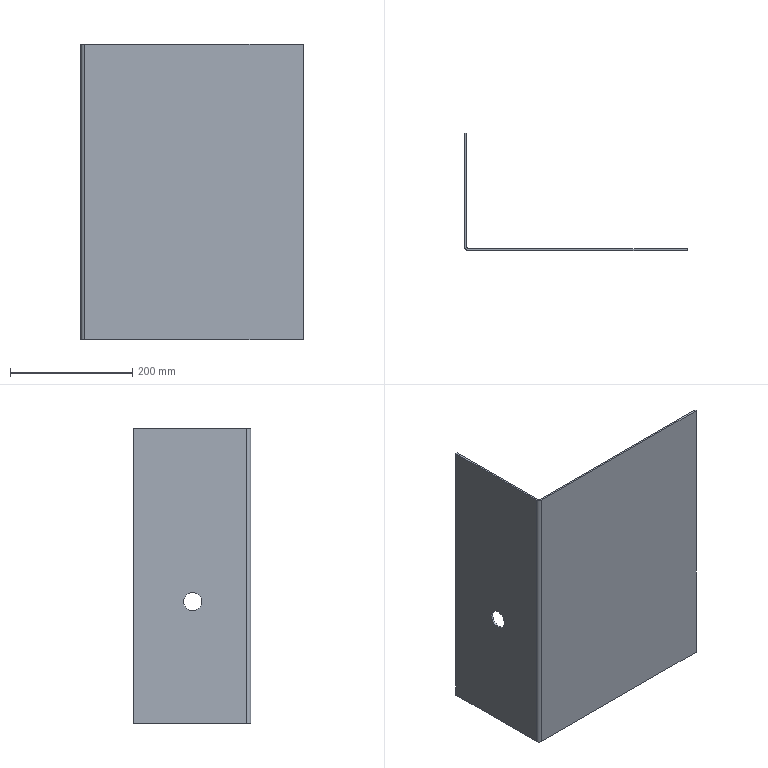Part | SolidWorks | features Cut 1, FlatPattern 1, SMBaseFlange 1, SheetMetal 1 | 1 solid | 16 faces | box 364 x 192 x 484 mm | volume 798031 mm3 | plane 12 | cylinder 4 | commonest cylinder face diameters 30 x2 6 x1 12 x1
STEP:
#1=CARTESIAN_POINT('',(3.,95.,215.));
#2=VERTEX_POINT('',#1);
#3=CARTESIAN_POINT('',(3.,95.,185.));
#4=VERTEX_POINT('',#3);
#5=CARTESIAN_POINT('',(3.,95.,200.));
#6=DIRECTION('',(1.,0.,0.));
#7=DIRECTION('',(0.,0.,-1.));
#8=AXIS2_PLACEMENT_3D('',#5,#6,#7);
#9=CIRCLE('',#8,15.);
#10=EDGE_CURVE('',#2,#4,#9,.T.);
#11=ORIENTED_EDGE('',*,*,#10,.T.);
#12=CARTESIAN_POINT('',(0.,95.,185.));
#13=VERTEX_POINT('',#12);
#14=CARTESIAN_POINT('',(10.,95.,185.));
#15=DIRECTION('',(-1.,0.,0.));
#16=VECTOR('',#15,1000.);
#17=LINE('',#14,#16);
#18=EDGE_CURVE('',#4,#13,#17,.T.);
#19=ORIENTED_EDGE('',*,*,#18,.T.);
#20=CARTESIAN_POINT('',(0.,95.,215.));
#21=VERTEX_POINT('',#20);
#22=CARTESIAN_POINT('',(0.,95.,200.));
#23=DIRECTION('',(-1.,0.,0.));
#24=DIRECTION('',(0.,0.,1.));
#25=AXIS2_PLACEMENT_3D('',#22,#23,#24);
#26=CIRCLE('',#25,15.);
#27=EDGE_CURVE('',#13,#21,#26,.T.);
#28=ORIENTED_EDGE('',*,*,#27,.T.);
#29=CARTESIAN_POINT('',(10.,95.,215.));
#30=DIRECTION('',(-1.,0.,0.));
#31=VECTOR('',#30,1000.);
#32=LINE('',#29,#31);
#33=EDGE_CURVE('',#2,#21,#32,.T.);
#34=ORIENTED_EDGE('',*,*,#33,.F.);
#35=EDGE_LOOP('',(#11,#19,#28,#34));
#36=FACE_OUTER_BOUND('',#35,.T.);
#37=CARTESIAN_POINT('',(10.,95.,200.));
#38=DIRECTION('',(-1.,0.,0.));
#39=DIRECTION('',(0.,0.,1.));
#40=AXIS2_PLACEMENT_3D('',#37,#38,#39);
#41=CYLINDRICAL_SURFACE('',#40,15.);
#42=ADVANCED_FACE('',(#36),#41,.F.);
#43=CARTESIAN_POINT('',(0.,6.,484.));
#44=VERTEX_POINT('',#43);
#45=CARTESIAN_POINT('',(3.,6.,484.));
#46=VERTEX_POINT('',#45);
#47=CARTESIAN_POINT('',(0.,6.,484.));
#48=DIRECTION('',(1.,0.,0.));
#49=VECTOR('',#48,1000.);
#50=LINE('',#47,#49);
#51=EDGE_CURVE('',#44,#46,#50,.T.);
#52=ORIENTED_EDGE('',*,*,#51,.F.);
#53=CARTESIAN_POINT('',(6.,0.,484.));
#54=VERTEX_POINT('',#53);
#55=CARTESIAN_POINT('',(6.,6.,484.));
#56=DIRECTION('',(0.,0.,1.));
#57=DIRECTION('',(-1.,0.,0.));
#58=AXIS2_PLACEMENT_3D('',#55,#56,#57);
#59=CIRCLE('',#58,6.);
#60=EDGE_CURVE('',#44,#54,#59,.T.);
#61=ORIENTED_EDGE('',*,*,#60,.T.);
#62=CARTESIAN_POINT('',(6.,3.,484.));
#63=VERTEX_POINT('',#62);
#64=CARTESIAN_POINT('',(6.,3.,484.));
#65=DIRECTION('',(0.,-1.,0.));
#66=VECTOR('',#65,1000.);
#67=LINE('',#64,#66);
#68=EDGE_CURVE('',#63,#54,#67,.T.);
#69=ORIENTED_EDGE('',*,*,#68,.F.);
#70=CARTESIAN_POINT('',(6.,6.,484.));
#71=DIRECTION('',(0.,0.,1.));
#72=DIRECTION('',(1.,0.,0.));
#73=AXIS2_PLACEMENT_3D('',#70,#71,#72);
#74=CIRCLE('',#73,3.);
#75=EDGE_CURVE('',#46,#63,#74,.T.);
#76=ORIENTED_EDGE('',*,*,#75,.F.);
#77=EDGE_LOOP('',(#52,#61,#69,#76));
#78=FACE_OUTER_BOUND('',#77,.T.);
#79=CARTESIAN_POINT('',(0.,6.,484.));
#80=DIRECTION('',(0.,0.,1.));
#81=DIRECTION('',(1.,0.,0.));
#82=AXIS2_PLACEMENT_3D('',#79,#80,#81);
#83=PLANE('',#82);
#84=ADVANCED_FACE('',(#78),#83,.T.);
#85=CARTESIAN_POINT('',(0.,192.,484.));
#86=VERTEX_POINT('',#85);
#87=CARTESIAN_POINT('',(0.,0.,484.));
#88=DIRECTION('',(0.,-1.,0.));
#89=VECTOR('',#88,1000.);
#90=LINE('',#87,#89);
#91=EDGE_CURVE('',#86,#44,#90,.T.);
#92=ORIENTED_EDGE('',*,*,#91,.T.);
#93=ORIENTED_EDGE('',*,*,#51,.T.);
#94=CARTESIAN_POINT('',(3.,192.,484.));
#95=VERTEX_POINT('',#94);
#96=CARTESIAN_POINT('',(3.,0.,484.));
#97=DIRECTION('',(0.,-1.,0.));
#98=VECTOR('',#97,1000.);
#99=LINE('',#96,#98);
#100=EDGE_CURVE('',#95,#46,#99,.T.);
#101=ORIENTED_EDGE('',*,*,#100,.F.);
#102=CARTESIAN_POINT('',(0.,192.,484.));
#103=DIRECTION('',(1.,0.,0.));
#104=VECTOR('',#103,1000.);
#105=LINE('',#102,#104);
#106=EDGE_CURVE('',#86,#95,#105,.T.);
#107=ORIENTED_EDGE('',*,*,#106,.F.);
#108=EDGE_LOOP('',(#92,#93,#101,#107));
#109=FACE_OUTER_BOUND('',#108,.T.);
#110=CARTESIAN_POINT('',(6.,3.,484.));
#111=DIRECTION('',(0.,0.,1.));
#112=DIRECTION('',(1.,0.,0.));
#113=AXIS2_PLACEMENT_3D('',#110,#111,#112);
#114=PLANE('',#113);
#115=ADVANCED_FACE('',(#109),#114,.T.);
#116=CARTESIAN_POINT('',(6.,0.,0.));
#117=VERTEX_POINT('',#116);
#118=CARTESIAN_POINT('',(6.,3.,0.));
#119=VERTEX_POINT('',#118);
#120=CARTESIAN_POINT('',(6.,0.,0.));
#121=DIRECTION('',(0.,1.,0.));
#122=VECTOR('',#121,1000.);
#123=LINE('',#120,#122);
#124=EDGE_CURVE('',#117,#119,#123,.T.);
#125=ORIENTED_EDGE('',*,*,#124,.F.);
#126=CARTESIAN_POINT('',(0.,6.,0.));
#127=VERTEX_POINT('',#126);
#128=CARTESIAN_POINT('',(6.,6.,0.));
#129=DIRECTION('',(0.,0.,1.));
#130=DIRECTION('',(-1.,0.,0.));
#131=AXIS2_PLACEMENT_3D('',#128,#129,#130);
#132=CIRCLE('',#131,6.);
#133=EDGE_CURVE('',#127,#117,#132,.T.);
#134=ORIENTED_EDGE('',*,*,#133,.F.);
#135=CARTESIAN_POINT('',(3.,6.,0.));
#136=VERTEX_POINT('',#135);
#137=CARTESIAN_POINT('',(3.,6.,0.));
#138=DIRECTION('',(-1.,0.,0.));
#139=VECTOR('',#138,1000.);
#140=LINE('',#137,#139);
#141=EDGE_CURVE('',#136,#127,#140,.T.);
#142=ORIENTED_EDGE('',*,*,#141,.F.);
#143=CARTESIAN_POINT('',(6.,6.,0.));
#144=DIRECTION('',(0.,0.,1.));
#145=DIRECTION('',(1.,0.,0.));
#146=AXIS2_PLACEMENT_3D('',#143,#144,#145);
#147=CIRCLE('',#146,3.);
#148=EDGE_CURVE('',#136,#119,#147,.T.);
#149=ORIENTED_EDGE('',*,*,#148,.T.);
#150=EDGE_LOOP('',(#125,#134,#142,#149));
#151=FACE_OUTER_BOUND('',#150,.T.);
#152=CARTESIAN_POINT('',(6.,0.,0.));
#153=DIRECTION('',(0.,0.,-1.));
#154=DIRECTION('',(-1.,0.,0.));
#155=AXIS2_PLACEMENT_3D('',#152,#153,#154);
#156=PLANE('',#155);
#157=ADVANCED_FACE('',(#151),#156,.T.);
#158=CARTESIAN_POINT('',(364.,0.,0.));
#159=VERTEX_POINT('',#158);
#160=CARTESIAN_POINT('',(0.,0.,0.));
#161=DIRECTION('',(1.,0.,0.));
#162=VECTOR('',#161,1000.);
#163=LINE('',#160,#162);
#164=EDGE_CURVE('',#117,#159,#163,.T.);
#165=ORIENTED_EDGE('',*,*,#164,.F.);
#166=ORIENTED_EDGE('',*,*,#124,.T.);
#167=CARTESIAN_POINT('',(364.,3.,0.));
#168=VERTEX_POINT('',#167);
#169=CARTESIAN_POINT('',(0.,3.,0.));
#170=DIRECTION('',(1.,0.,0.));
#171=VECTOR('',#170,1000.);
#172=LINE('',#169,#171);
#173=EDGE_CURVE('',#119,#168,#172,.T.);
#174=ORIENTED_EDGE('',*,*,#173,.T.);
#175=CARTESIAN_POINT('',(364.,3.,0.));
#176=DIRECTION('',(0.,-1.,0.));
#177=VECTOR('',#176,1000.);
#178=LINE('',#175,#177);
#179=EDGE_CURVE('',#168,#159,#178,.T.);
#180=ORIENTED_EDGE('',*,*,#179,.T.);
#181=EDGE_LOOP('',(#165,#166,#174,#180));
#182=FACE_OUTER_BOUND('',#181,.T.);
#183=CARTESIAN_POINT('',(3.,6.,0.));
#184=DIRECTION('',(0.,0.,-1.));
#185=DIRECTION('',(-1.,0.,0.));
#186=AXIS2_PLACEMENT_3D('',#183,#184,#185);
#187=PLANE('',#186);
#188=ADVANCED_FACE('',(#182),#187,.T.);
#189=ORIENTED_EDGE('',*,*,#164,.T.);
#190=CARTESIAN_POINT('',(364.,0.,484.));
#191=VERTEX_POINT('',#190);
#192=CARTESIAN_POINT('',(364.,0.,484.));
#193=DIRECTION('',(0.,0.,-1.));
#194=VECTOR('',#193,1000.);
#195=LINE('',#192,#194);
#196=EDGE_CURVE('',#191,#159,#195,.T.);
#197=ORIENTED_EDGE('',*,*,#196,.F.);
#198=CARTESIAN_POINT('',(0.,0.,484.));
#199=DIRECTION('',(1.,0.,0.));
#200=VECTOR('',#199,1000.);
#201=LINE('',#198,#200);
#202=EDGE_CURVE('',#54,#191,#201,.T.);
#203=ORIENTED_EDGE('',*,*,#202,.F.);
#204=CARTESIAN_POINT('',(6.,0.,484.));
#205=DIRECTION('',(0.,0.,-1.));
#206=VECTOR('',#205,1000.);
#207=LINE('',#204,#206);
#208=EDGE_CURVE('',#54,#117,#207,.T.);
#209=ORIENTED_EDGE('',*,*,#208,.T.);
#210=EDGE_LOOP('',(#189,#197,#203,#209));
#211=FACE_OUTER_BOUND('',#210,.T.);
#212=CARTESIAN_POINT('',(0.,0.,484.));
#213=DIRECTION('',(0.,1.,0.));
#214=DIRECTION('',(0.,0.,1.));
#215=AXIS2_PLACEMENT_3D('',#212,#213,#214);
#216=PLANE('',#215);
#217=ADVANCED_FACE('',(#211),#216,.F.);
#218=ORIENTED_EDGE('',*,*,#179,.F.);
#219=CARTESIAN_POINT('',(364.,3.,484.));
#220=VERTEX_POINT('',#219);
#221=CARTESIAN_POINT('',(364.,3.,484.));
#222=DIRECTION('',(0.,0.,-1.));
#223=VECTOR('',#222,1000.);
#224=LINE('',#221,#223);
#225=EDGE_CURVE('',#220,#168,#224,.T.);
#226=ORIENTED_EDGE('',*,*,#225,.F.);
#227=CARTESIAN_POINT('',(364.,3.,484.));
#228=DIRECTION('',(0.,-1.,0.));
#229=VECTOR('',#228,1000.);
#230=LINE('',#227,#229);
#231=EDGE_CURVE('',#220,#191,#230,.T.);
#232=ORIENTED_EDGE('',*,*,#231,.T.);
#233=ORIENTED_EDGE('',*,*,#196,.T.);
#234=EDGE_LOOP('',(#218,#226,#232,#233));
#235=FACE_OUTER_BOUND('',#234,.T.);
#236=CARTESIAN_POINT('',(364.,3.,484.));
#237=DIRECTION('',(1.,0.,0.));
#238=DIRECTION('',(0.,0.,-1.));
#239=AXIS2_PLACEMENT_3D('',#236,#237,#238);
#240=PLANE('',#239);
#241=ADVANCED_FACE('',(#235),#240,.T.);
#242=ORIENTED_EDGE('',*,*,#173,.F.);
#243=CARTESIAN_POINT('',(6.,3.,484.));
#244=DIRECTION('',(0.,0.,-1.));
#245=VECTOR('',#244,1000.);
#246=LINE('',#243,#245);
#247=EDGE_CURVE('',#63,#119,#246,.T.);
#248=ORIENTED_EDGE('',*,*,#247,.F.);
#249=CARTESIAN_POINT('',(0.,3.,484.));
#250=DIRECTION('',(1.,0.,0.));
#251=VECTOR('',#250,1000.);
#252=LINE('',#249,#251);
#253=EDGE_CURVE('',#63,#220,#252,.T.);
#254=ORIENTED_EDGE('',*,*,#253,.T.);
#255=ORIENTED_EDGE('',*,*,#225,.T.);
#256=EDGE_LOOP('',(#242,#248,#254,#255));
#257=FACE_OUTER_BOUND('',#256,.T.);
#258=CARTESIAN_POINT('',(0.,3.,484.));
#259=DIRECTION('',(0.,1.,0.));
#260=DIRECTION('',(0.,0.,1.));
#261=AXIS2_PLACEMENT_3D('',#258,#259,#260);
#262=PLANE('',#261);
#263=ADVANCED_FACE('',(#257),#262,.T.);
#264=ORIENTED_EDGE('',*,*,#148,.F.);
#265=CARTESIAN_POINT('',(3.,6.,484.));
#266=DIRECTION('',(0.,0.,-1.));
#267=VECTOR('',#266,1000.);
#268=LINE('',#265,#267);
#269=EDGE_CURVE('',#46,#136,#268,.T.);
#270=ORIENTED_EDGE('',*,*,#269,.F.);
#271=ORIENTED_EDGE('',*,*,#75,.T.);
#272=ORIENTED_EDGE('',*,*,#247,.T.);
#273=EDGE_LOOP('',(#264,#270,#271,#272));
#274=FACE_OUTER_BOUND('',#273,.T.);
#275=CARTESIAN_POINT('',(6.,6.,484.));
#276=DIRECTION('',(0.,0.,-1.));
#277=DIRECTION('',(-1.,0.,0.));
#278=AXIS2_PLACEMENT_3D('',#275,#276,#277);
#279=CYLINDRICAL_SURFACE('',#278,3.);
#280=ADVANCED_FACE('',(#274),#279,.F.);
#281=ORIENTED_EDGE('',*,*,#10,.F.);
#282=CARTESIAN_POINT('',(3.,95.,200.));
#283=DIRECTION('',(1.,0.,0.));
#284=DIRECTION('',(0.,0.,-1.));
#285=AXIS2_PLACEMENT_3D('',#282,#283,#284);
#286=CIRCLE('',#285,15.);
#287=EDGE_CURVE('',#4,#2,#286,.T.);
#288=ORIENTED_EDGE('',*,*,#287,.F.);
#289=EDGE_LOOP('',(#281,#288));
#290=FACE_BOUND('',#289,.T.);
#291=CARTESIAN_POINT('',(3.,192.,0.));
#292=VERTEX_POINT('',#291);
#293=CARTESIAN_POINT('',(3.,0.,0.));
#294=DIRECTION('',(0.,-1.,0.));
#295=VECTOR('',#294,1000.);
#296=LINE('',#293,#295);
#297=EDGE_CURVE('',#292,#136,#296,.T.);
#298=ORIENTED_EDGE('',*,*,#297,.F.);
#299=CARTESIAN_POINT('',(3.,192.,484.));
#300=DIRECTION('',(0.,0.,-1.));
#301=VECTOR('',#300,1000.);
#302=LINE('',#299,#301);
#303=EDGE_CURVE('',#95,#292,#302,.T.);
#304=ORIENTED_EDGE('',*,*,#303,.F.);
#305=ORIENTED_EDGE('',*,*,#100,.T.);
#306=ORIENTED_EDGE('',*,*,#269,.T.);
#307=EDGE_LOOP('',(#298,#304,#305,#306));
#308=FACE_OUTER_BOUND('',#307,.T.);
#309=CARTESIAN_POINT('',(3.,0.,484.));
#310=DIRECTION('',(1.,0.,0.));
#311=DIRECTION('',(0.,0.,-1.));
#312=AXIS2_PLACEMENT_3D('',#309,#310,#311);
#313=PLANE('',#312);
#314=ADVANCED_FACE('',(#290,#308),#313,.T.);
#315=CARTESIAN_POINT('',(0.,192.,0.));
#316=VERTEX_POINT('',#315);
#317=CARTESIAN_POINT('',(0.,192.,0.));
#318=DIRECTION('',(1.,0.,0.));
#319=VECTOR('',#318,1000.);
#320=LINE('',#317,#319);
#321=EDGE_CURVE('',#316,#292,#320,.T.);
#322=ORIENTED_EDGE('',*,*,#321,.F.);
#323=CARTESIAN_POINT('',(0.,192.,484.));
#324=DIRECTION('',(0.,0.,-1.));
#325=VECTOR('',#324,1000.);
#326=LINE('',#323,#325);
#327=EDGE_CURVE('',#86,#316,#326,.T.);
#328=ORIENTED_EDGE('',*,*,#327,.F.);
#329=ORIENTED_EDGE('',*,*,#106,.T.);
#330=ORIENTED_EDGE('',*,*,#303,.T.);
#331=EDGE_LOOP('',(#322,#328,#329,#330));
#332=FACE_OUTER_BOUND('',#331,.T.);
#333=CARTESIAN_POINT('',(0.,192.,484.));
#334=DIRECTION('',(0.,1.,0.));
#335=DIRECTION('',(0.,0.,1.));
#336=AXIS2_PLACEMENT_3D('',#333,#334,#335);
#337=PLANE('',#336);
#338=ADVANCED_FACE('',(#332),#337,.T.);
#339=CARTESIAN_POINT('',(0.,95.,200.));
#340=DIRECTION('',(-1.,0.,0.));
#341=DIRECTION('',(0.,0.,1.));
#342=AXIS2_PLACEMENT_3D('',#339,#340,#341);
#343=CIRCLE('',#342,15.);
#344=EDGE_CURVE('',#21,#13,#343,.T.);
#345=ORIENTED_EDGE('',*,*,#344,.F.);
#346=ORIENTED_EDGE('',*,*,#27,.F.);
#347=EDGE_LOOP('',(#345,#346));
#348=FACE_BOUND('',#347,.T.);
#349=CARTESIAN_POINT('',(0.,0.,0.));
#350=DIRECTION('',(0.,-1.,0.));
#351=VECTOR('',#350,1000.);
#352=LINE('',#349,#351);
#353=EDGE_CURVE('',#316,#127,#352,.T.);
#354=ORIENTED_EDGE('',*,*,#353,.T.);
#355=CARTESIAN_POINT('',(0.,6.,484.));
#356=DIRECTION('',(0.,0.,-1.));
#357=VECTOR('',#356,1000.);
#358=LINE('',#355,#357);
#359=EDGE_CURVE('',#44,#127,#358,.T.);
#360=ORIENTED_EDGE('',*,*,#359,.F.);
#361=ORIENTED_EDGE('',*,*,#91,.F.);
#362=ORIENTED_EDGE('',*,*,#327,.T.);
#363=EDGE_LOOP('',(#354,#360,#361,#362));
#364=FACE_OUTER_BOUND('',#363,.T.);
#365=CARTESIAN_POINT('',(0.,0.,484.));
#366=DIRECTION('',(1.,0.,0.));
#367=DIRECTION('',(0.,0.,-1.));
#368=AXIS2_PLACEMENT_3D('',#365,#366,#367);
#369=PLANE('',#368);
#370=ADVANCED_FACE('',(#348,#364),#369,.F.);
#371=ORIENTED_EDGE('',*,*,#133,.T.);
#372=ORIENTED_EDGE('',*,*,#208,.F.);
#373=ORIENTED_EDGE('',*,*,#60,.F.);
#374=ORIENTED_EDGE('',*,*,#359,.T.);
#375=EDGE_LOOP('',(#371,#372,#373,#374));
#376=FACE_OUTER_BOUND('',#375,.T.);
#377=CARTESIAN_POINT('',(6.,6.,484.));
#378=DIRECTION('',(0.,0.,-1.));
#379=DIRECTION('',(-1.,0.,0.));
#380=AXIS2_PLACEMENT_3D('',#377,#378,#379);
#381=CYLINDRICAL_SURFACE('',#380,6.);
#382=ADVANCED_FACE('',(#376),#381,.T.);
#383=ORIENTED_EDGE('',*,*,#202,.T.);
#384=ORIENTED_EDGE('',*,*,#231,.F.);
#385=ORIENTED_EDGE('',*,*,#253,.F.);
#386=ORIENTED_EDGE('',*,*,#68,.T.);
#387=EDGE_LOOP('',(#383,#384,#385,#386));
#388=FACE_OUTER_BOUND('',#387,.T.);
#389=CARTESIAN_POINT('',(6.,6.,484.));
#390=DIRECTION('',(0.,0.,1.));
#391=DIRECTION('',(1.,0.,0.));
#392=AXIS2_PLACEMENT_3D('',#389,#390,#391);
#393=PLANE('',#392);
#394=ADVANCED_FACE('',(#388),#393,.T.);
#395=ORIENTED_EDGE('',*,*,#297,.T.);
#396=ORIENTED_EDGE('',*,*,#141,.T.);
#397=ORIENTED_EDGE('',*,*,#353,.F.);
#398=ORIENTED_EDGE('',*,*,#321,.T.);
#399=EDGE_LOOP('',(#395,#396,#397,#398));
#400=FACE_OUTER_BOUND('',#399,.T.);
#401=CARTESIAN_POINT('',(6.,6.,0.));
#402=DIRECTION('',(0.,0.,1.));
#403=DIRECTION('',(1.,0.,0.));
#404=AXIS2_PLACEMENT_3D('',#401,#402,#403);
#405=PLANE('',#404);
#406=ADVANCED_FACE('',(#400),#405,.F.);
#407=ORIENTED_EDGE('',*,*,#18,.F.);
#408=ORIENTED_EDGE('',*,*,#287,.T.);
#409=ORIENTED_EDGE('',*,*,#33,.T.);
#410=ORIENTED_EDGE('',*,*,#344,.T.);
#411=EDGE_LOOP('',(#407,#408,#409,#410));
#412=FACE_OUTER_BOUND('',#411,.T.);
#413=CARTESIAN_POINT('',(10.,95.,200.));
#414=DIRECTION('',(-1.,0.,0.));
#415=DIRECTION('',(0.,0.,1.));
#416=AXIS2_PLACEMENT_3D('',#413,#414,#415);
#417=CYLINDRICAL_SURFACE('',#416,15.);
#418=ADVANCED_FACE('',(#412),#417,.F.);
#419=CLOSED_SHELL('',(#42,#84,#115,#157,#188,#217,#241,#263,#280,#314,#338,#370,#382,#394,#406,#418));
#420=MANIFOLD_SOLID_BREP('',#419);
#421=CARTESIAN_POINT('',(0.,0.,0.));
#422=DIRECTION('',(0.,0.,1.));
#423=DIRECTION('',(1.,0.,0.));
#424=AXIS2_PLACEMENT_3D('',#421,#422,#423);
#425=(LENGTH_UNIT()NAMED_UNIT(*)SI_UNIT(.MILLI.,.METRE.));
#426=UNCERTAINTY_MEASURE_WITH_UNIT(LENGTH_MEASURE(0.00001),#425,'','');
#427=(NAMED_UNIT(*)PLANE_ANGLE_UNIT()SI_UNIT($,.RADIAN.));
#428=(NAMED_UNIT(*)SI_UNIT($,.STERADIAN.)SOLID_ANGLE_UNIT());
#429=(GEOMETRIC_REPRESENTATION_CONTEXT(3)GLOBAL_UNCERTAINTY_ASSIGNED_CONTEXT((#426))GLOBAL_UNIT_ASSIGNED_CONTEXT((#425,#427,#428))REPRESENTATION_CONTEXT('',''));
#430=ADVANCED_BREP_SHAPE_REPRESENTATION('',(#420,#424),#429);